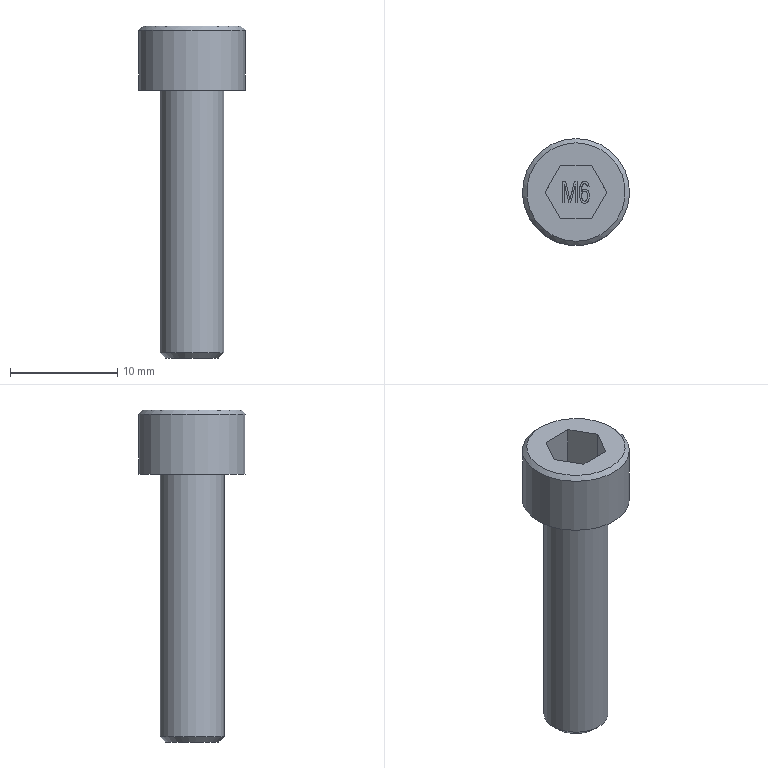Part | STEP file | EM10602500 | 1 solid | 38 faces | box 10 x 10 x 31 mm | volume 1087 mm3 | plane 25 | other 9 | cylinder 2 | cone 2 | commonest cylinder face diameters 6 x1 10 x1